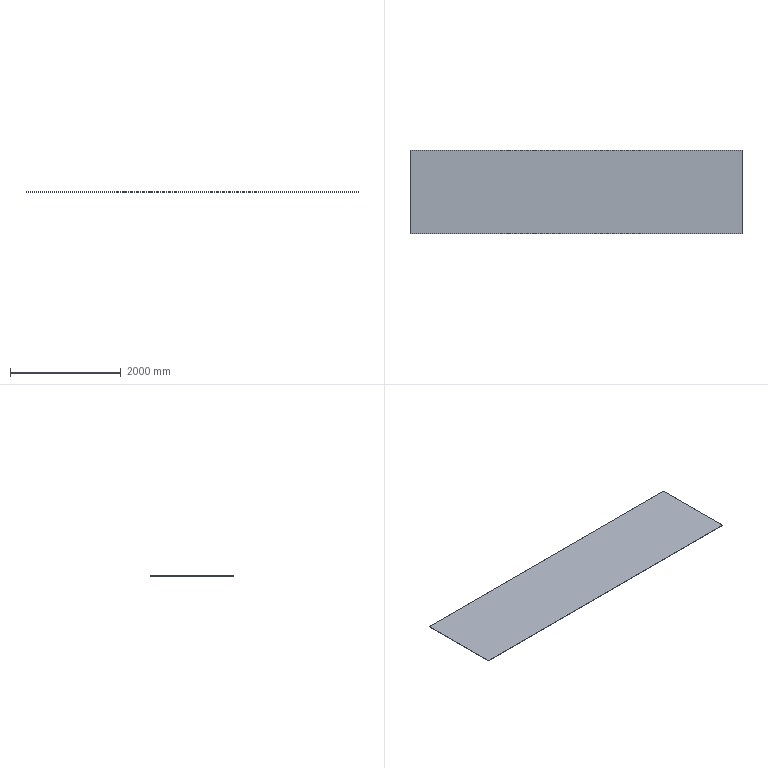Part | SolidWorks | features Extrusion 1 | 1 solid | 6 faces | box 6000 x 1510 x 6 mm | volume 54360000 mm3 | plane 6
STEP:
#1=CARTESIAN_POINT('',(0.,1510.,0.));
#2=VERTEX_POINT('',#1);
#3=CARTESIAN_POINT('',(0.,0.,0.));
#4=VERTEX_POINT('',#3);
#5=CARTESIAN_POINT('',(0.,0.,0.));
#6=DIRECTION('',(0.,-1.,0.));
#7=VECTOR('',#6,1000.);
#8=LINE('',#5,#7);
#9=EDGE_CURVE('',#2,#4,#8,.T.);
#10=ORIENTED_EDGE('',*,*,#9,.T.);
#11=CARTESIAN_POINT('',(0.,0.,6.));
#12=VERTEX_POINT('',#11);
#13=CARTESIAN_POINT('',(0.,0.,6.));
#14=DIRECTION('',(0.,0.,-1.));
#15=VECTOR('',#14,1000.);
#16=LINE('',#13,#15);
#17=EDGE_CURVE('',#12,#4,#16,.T.);
#18=ORIENTED_EDGE('',*,*,#17,.F.);
#19=CARTESIAN_POINT('',(0.,1510.,6.));
#20=VERTEX_POINT('',#19);
#21=CARTESIAN_POINT('',(0.,0.,6.));
#22=DIRECTION('',(0.,-1.,0.));
#23=VECTOR('',#22,1000.);
#24=LINE('',#21,#23);
#25=EDGE_CURVE('',#20,#12,#24,.T.);
#26=ORIENTED_EDGE('',*,*,#25,.F.);
#27=CARTESIAN_POINT('',(0.,1510.,6.));
#28=DIRECTION('',(0.,0.,-1.));
#29=VECTOR('',#28,1000.);
#30=LINE('',#27,#29);
#31=EDGE_CURVE('',#20,#2,#30,.T.);
#32=ORIENTED_EDGE('',*,*,#31,.T.);
#33=EDGE_LOOP('',(#10,#18,#26,#32));
#34=FACE_OUTER_BOUND('',#33,.T.);
#35=CARTESIAN_POINT('',(0.,0.,6.));
#36=DIRECTION('',(1.,0.,0.));
#37=DIRECTION('',(0.,0.,-1.));
#38=AXIS2_PLACEMENT_3D('',#35,#36,#37);
#39=PLANE('',#38);
#40=ADVANCED_FACE('',(#34),#39,.F.);
#41=CARTESIAN_POINT('',(6000.,0.,0.));
#42=VERTEX_POINT('',#41);
#43=CARTESIAN_POINT('',(0.,0.,0.));
#44=DIRECTION('',(1.,0.,0.));
#45=VECTOR('',#44,1000.);
#46=LINE('',#43,#45);
#47=EDGE_CURVE('',#4,#42,#46,.T.);
#48=ORIENTED_EDGE('',*,*,#47,.T.);
#49=CARTESIAN_POINT('',(6000.,0.,6.));
#50=VERTEX_POINT('',#49);
#51=CARTESIAN_POINT('',(6000.,0.,6.));
#52=DIRECTION('',(0.,0.,-1.));
#53=VECTOR('',#52,1000.);
#54=LINE('',#51,#53);
#55=EDGE_CURVE('',#50,#42,#54,.T.);
#56=ORIENTED_EDGE('',*,*,#55,.F.);
#57=CARTESIAN_POINT('',(0.,0.,6.));
#58=DIRECTION('',(1.,0.,0.));
#59=VECTOR('',#58,1000.);
#60=LINE('',#57,#59);
#61=EDGE_CURVE('',#12,#50,#60,.T.);
#62=ORIENTED_EDGE('',*,*,#61,.F.);
#63=ORIENTED_EDGE('',*,*,#17,.T.);
#64=EDGE_LOOP('',(#48,#56,#62,#63));
#65=FACE_OUTER_BOUND('',#64,.T.);
#66=CARTESIAN_POINT('',(0.,0.,6.));
#67=DIRECTION('',(0.,1.,0.));
#68=DIRECTION('',(0.,0.,1.));
#69=AXIS2_PLACEMENT_3D('',#66,#67,#68);
#70=PLANE('',#69);
#71=ADVANCED_FACE('',(#65),#70,.F.);
#72=CARTESIAN_POINT('',(6000.,1510.,0.));
#73=VERTEX_POINT('',#72);
#74=CARTESIAN_POINT('',(6000.,0.,0.));
#75=DIRECTION('',(0.,1.,0.));
#76=VECTOR('',#75,1000.);
#77=LINE('',#74,#76);
#78=EDGE_CURVE('',#42,#73,#77,.T.);
#79=ORIENTED_EDGE('',*,*,#78,.T.);
#80=CARTESIAN_POINT('',(6000.,1510.,6.));
#81=VERTEX_POINT('',#80);
#82=CARTESIAN_POINT('',(6000.,1510.,6.));
#83=DIRECTION('',(0.,0.,-1.));
#84=VECTOR('',#83,1000.);
#85=LINE('',#82,#84);
#86=EDGE_CURVE('',#81,#73,#85,.T.);
#87=ORIENTED_EDGE('',*,*,#86,.F.);
#88=CARTESIAN_POINT('',(6000.,0.,6.));
#89=DIRECTION('',(0.,1.,0.));
#90=VECTOR('',#89,1000.);
#91=LINE('',#88,#90);
#92=EDGE_CURVE('',#50,#81,#91,.T.);
#93=ORIENTED_EDGE('',*,*,#92,.F.);
#94=ORIENTED_EDGE('',*,*,#55,.T.);
#95=EDGE_LOOP('',(#79,#87,#93,#94));
#96=FACE_OUTER_BOUND('',#95,.T.);
#97=CARTESIAN_POINT('',(6000.,0.,6.));
#98=DIRECTION('',(-1.,0.,0.));
#99=DIRECTION('',(0.,0.,1.));
#100=AXIS2_PLACEMENT_3D('',#97,#98,#99);
#101=PLANE('',#100);
#102=ADVANCED_FACE('',(#96),#101,.F.);
#103=CARTESIAN_POINT('',(0.,1510.,0.));
#104=DIRECTION('',(-1.,0.,0.));
#105=VECTOR('',#104,1000.);
#106=LINE('',#103,#105);
#107=EDGE_CURVE('',#73,#2,#106,.T.);
#108=ORIENTED_EDGE('',*,*,#107,.T.);
#109=ORIENTED_EDGE('',*,*,#31,.F.);
#110=CARTESIAN_POINT('',(0.,1510.,6.));
#111=DIRECTION('',(-1.,0.,0.));
#112=VECTOR('',#111,1000.);
#113=LINE('',#110,#112);
#114=EDGE_CURVE('',#81,#20,#113,.T.);
#115=ORIENTED_EDGE('',*,*,#114,.F.);
#116=ORIENTED_EDGE('',*,*,#86,.T.);
#117=EDGE_LOOP('',(#108,#109,#115,#116));
#118=FACE_OUTER_BOUND('',#117,.T.);
#119=CARTESIAN_POINT('',(0.,1510.,6.));
#120=DIRECTION('',(0.,-1.,0.));
#121=DIRECTION('',(0.,0.,-1.));
#122=AXIS2_PLACEMENT_3D('',#119,#120,#121);
#123=PLANE('',#122);
#124=ADVANCED_FACE('',(#118),#123,.F.);
#125=ORIENTED_EDGE('',*,*,#25,.T.);
#126=ORIENTED_EDGE('',*,*,#61,.T.);
#127=ORIENTED_EDGE('',*,*,#92,.T.);
#128=ORIENTED_EDGE('',*,*,#114,.T.);
#129=EDGE_LOOP('',(#125,#126,#127,#128));
#130=FACE_OUTER_BOUND('',#129,.T.);
#131=CARTESIAN_POINT('',(0.,0.,6.));
#132=DIRECTION('',(0.,0.,-1.));
#133=DIRECTION('',(-1.,0.,0.));
#134=AXIS2_PLACEMENT_3D('',#131,#132,#133);
#135=PLANE('',#134);
#136=ADVANCED_FACE('',(#130),#135,.F.);
#137=ORIENTED_EDGE('',*,*,#9,.F.);
#138=ORIENTED_EDGE('',*,*,#107,.F.);
#139=ORIENTED_EDGE('',*,*,#78,.F.);
#140=ORIENTED_EDGE('',*,*,#47,.F.);
#141=EDGE_LOOP('',(#137,#138,#139,#140));
#142=FACE_OUTER_BOUND('',#141,.T.);
#143=CARTESIAN_POINT('',(0.,0.,0.));
#144=DIRECTION('',(0.,0.,-1.));
#145=DIRECTION('',(-1.,0.,0.));
#146=AXIS2_PLACEMENT_3D('',#143,#144,#145);
#147=PLANE('',#146);
#148=ADVANCED_FACE('',(#142),#147,.T.);
#149=CLOSED_SHELL('',(#40,#71,#102,#124,#136,#148));
#150=MANIFOLD_SOLID_BREP('',#149);
#151=CARTESIAN_POINT('',(0.,0.,0.));
#152=DIRECTION('',(0.,0.,1.));
#153=DIRECTION('',(1.,0.,0.));
#154=AXIS2_PLACEMENT_3D('',#151,#152,#153);
#155=(LENGTH_UNIT()NAMED_UNIT(*)SI_UNIT(.MILLI.,.METRE.));
#156=UNCERTAINTY_MEASURE_WITH_UNIT(LENGTH_MEASURE(0.00001),#155,'','');
#157=(NAMED_UNIT(*)PLANE_ANGLE_UNIT()SI_UNIT($,.RADIAN.));
#158=(NAMED_UNIT(*)SI_UNIT($,.STERADIAN.)SOLID_ANGLE_UNIT());
#159=(GEOMETRIC_REPRESENTATION_CONTEXT(3)GLOBAL_UNCERTAINTY_ASSIGNED_CONTEXT((#156))GLOBAL_UNIT_ASSIGNED_CONTEXT((#155,#157,#158))REPRESENTATION_CONTEXT('',''));
#160=ADVANCED_BREP_SHAPE_REPRESENTATION('',(#150,#154),#159);